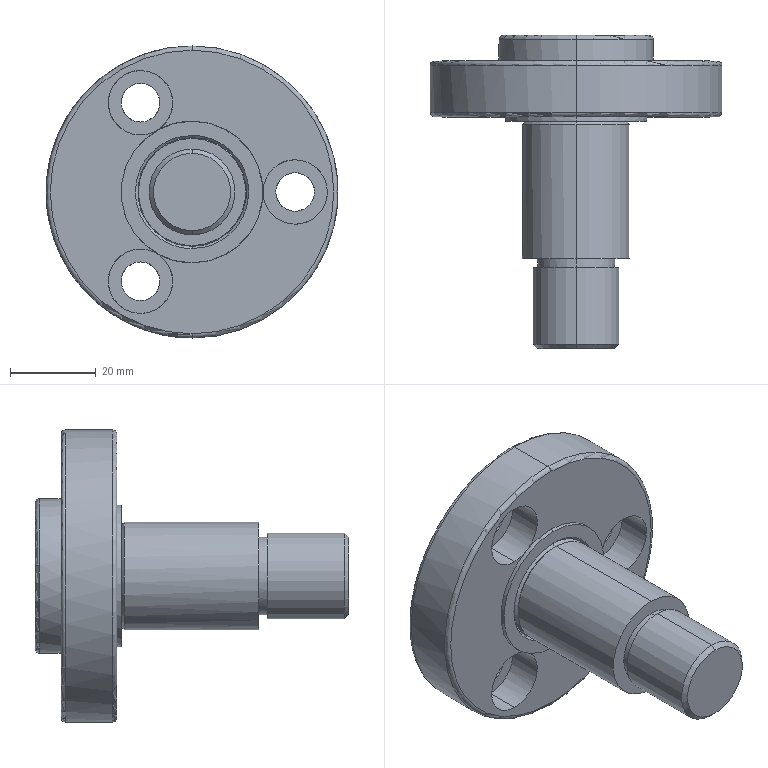Part | STEP file | 101000007742 | 1 solid | 48 faces | box 68 x 72.975 x 68 mm | volume 70977 mm3 | cylinder 24 | plane 10 | cone 8 | torus 6 | commonest cylinder face diameters 9 x6 15 x6 18 x2 20 x2 25 x2 33 x2